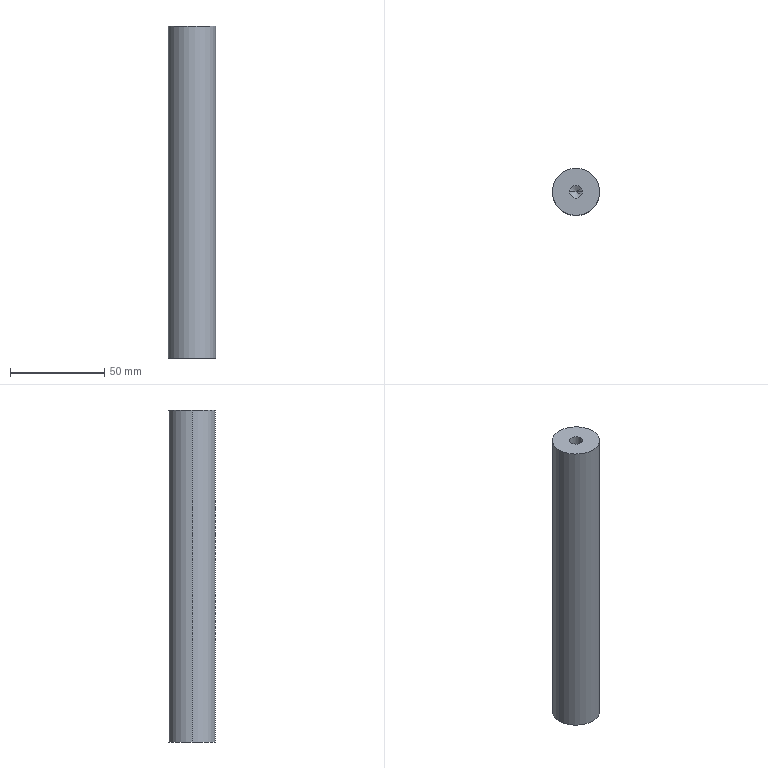Part | SolidWorks | features HoleWzd 2, Extrusion 1 | 1 solid | 12 faces | box 25 x 25 x 176 mm | volume 84910 mm3 | cylinder 6 | cone 4 | plane 2 | commonest cylinder face diameters 6.8 x4 25 x2
STEP:
#1=CARTESIAN_POINT('',(-3.4,0.,156.25));
#2=VERTEX_POINT('',#1);
#3=CARTESIAN_POINT('',(3.4,0.,156.25));
#4=VERTEX_POINT('',#3);
#5=CARTESIAN_POINT('',(0.,0.,156.25));
#6=DIRECTION('',(0.,0.,1.));
#7=DIRECTION('',(1.,0.,0.));
#8=AXIS2_PLACEMENT_3D('',#5,#6,#7);
#9=CIRCLE('',#8,3.4);
#10=EDGE_CURVE('',#2,#4,#9,.T.);
#11=ORIENTED_EDGE('',*,*,#10,.F.);
#12=CARTESIAN_POINT('',(-3.4,0.,176.));
#13=VERTEX_POINT('',#12);
#14=CARTESIAN_POINT('',(-3.4,0.,176.));
#15=DIRECTION('',(0.,0.,1.));
#16=VECTOR('',#15,1000.);
#17=LINE('',#14,#16);
#18=EDGE_CURVE('',#2,#13,#17,.T.);
#19=ORIENTED_EDGE('',*,*,#18,.T.);
#20=CARTESIAN_POINT('',(3.4,0.,176.));
#21=VERTEX_POINT('',#20);
#22=CARTESIAN_POINT('',(0.,0.,176.));
#23=DIRECTION('',(0.,0.,1.));
#24=DIRECTION('',(1.,0.,0.));
#25=AXIS2_PLACEMENT_3D('',#22,#23,#24);
#26=CIRCLE('',#25,3.4);
#27=EDGE_CURVE('',#13,#21,#26,.T.);
#28=ORIENTED_EDGE('',*,*,#27,.T.);
#29=CARTESIAN_POINT('',(3.4,0.,176.));
#30=DIRECTION('',(0.,0.,1.));
#31=VECTOR('',#30,1000.);
#32=LINE('',#29,#31);
#33=EDGE_CURVE('',#4,#21,#32,.T.);
#34=ORIENTED_EDGE('',*,*,#33,.F.);
#35=EDGE_LOOP('',(#11,#19,#28,#34));
#36=FACE_OUTER_BOUND('',#35,.T.);
#37=CARTESIAN_POINT('',(0.,0.,176.));
#38=DIRECTION('',(0.,0.,1.));
#39=DIRECTION('',(1.,0.,0.));
#40=AXIS2_PLACEMENT_3D('',#37,#38,#39);
#41=CYLINDRICAL_SURFACE('',#40,3.4);
#42=ADVANCED_FACE('',(#36),#41,.F.);
#43=CARTESIAN_POINT('',(0.,0.,154.207));
#44=VERTEX_POINT('',#43);
#45=CARTESIAN_POINT('',(3.4,0.,156.25));
#46=DIRECTION('',(0.8572,0.,0.515));
#47=VECTOR('',#46,1000.);
#48=LINE('',#45,#47);
#49=EDGE_CURVE('',#44,#4,#48,.T.);
#50=ORIENTED_EDGE('',*,*,#49,.F.);
#51=CARTESIAN_POINT('',(-3.4,0.,156.25));
#52=DIRECTION('',(-0.8572,0.,0.515));
#53=VECTOR('',#52,1000.);
#54=LINE('',#51,#53);
#55=EDGE_CURVE('',#44,#2,#54,.T.);
#56=ORIENTED_EDGE('',*,*,#55,.T.);
#57=ORIENTED_EDGE('',*,*,#10,.T.);
#58=EDGE_LOOP('',(#50,#56,#57));
#59=FACE_OUTER_BOUND('',#58,.T.);
#60=CARTESIAN_POINT('',(0.,0.,156.25));
#61=DIRECTION('',(0.,0.,1.));
#62=DIRECTION('',(1.,0.,0.));
#63=AXIS2_PLACEMENT_3D('',#60,#61,#62);
#64=CONICAL_SURFACE('',#63,3.4,1.03);
#65=ADVANCED_FACE('',(#59),#64,.F.);
#66=CARTESIAN_POINT('',(3.4,0.,19.75));
#67=VERTEX_POINT('',#66);
#68=CARTESIAN_POINT('',(-3.4,0.,19.75));
#69=VERTEX_POINT('',#68);
#70=CARTESIAN_POINT('',(0.,0.,19.75));
#71=DIRECTION('',(0.,0.,-1.));
#72=DIRECTION('',(-1.,0.,0.));
#73=AXIS2_PLACEMENT_3D('',#70,#71,#72);
#74=CIRCLE('',#73,3.4);
#75=EDGE_CURVE('',#67,#69,#74,.T.);
#76=ORIENTED_EDGE('',*,*,#75,.F.);
#77=CARTESIAN_POINT('',(3.4,0.,0.));
#78=VERTEX_POINT('',#77);
#79=CARTESIAN_POINT('',(3.4,0.,0.));
#80=DIRECTION('',(0.,0.,-1.));
#81=VECTOR('',#80,1000.);
#82=LINE('',#79,#81);
#83=EDGE_CURVE('',#67,#78,#82,.T.);
#84=ORIENTED_EDGE('',*,*,#83,.T.);
#85=CARTESIAN_POINT('',(-3.4,0.,0.));
#86=VERTEX_POINT('',#85);
#87=CARTESIAN_POINT('',(0.,0.,0.));
#88=DIRECTION('',(0.,0.,-1.));
#89=DIRECTION('',(-1.,0.,0.));
#90=AXIS2_PLACEMENT_3D('',#87,#88,#89);
#91=CIRCLE('',#90,3.4);
#92=EDGE_CURVE('',#78,#86,#91,.T.);
#93=ORIENTED_EDGE('',*,*,#92,.T.);
#94=CARTESIAN_POINT('',(-3.4,0.,0.));
#95=DIRECTION('',(0.,0.,-1.));
#96=VECTOR('',#95,1000.);
#97=LINE('',#94,#96);
#98=EDGE_CURVE('',#69,#86,#97,.T.);
#99=ORIENTED_EDGE('',*,*,#98,.F.);
#100=EDGE_LOOP('',(#76,#84,#93,#99));
#101=FACE_OUTER_BOUND('',#100,.T.);
#102=CARTESIAN_POINT('',(0.,0.,0.));
#103=DIRECTION('',(0.,0.,-1.));
#104=DIRECTION('',(-1.,0.,0.));
#105=AXIS2_PLACEMENT_3D('',#102,#103,#104);
#106=CYLINDRICAL_SURFACE('',#105,3.4);
#107=ADVANCED_FACE('',(#101),#106,.F.);
#108=CARTESIAN_POINT('',(0.,0.,21.793));
#109=VERTEX_POINT('',#108);
#110=CARTESIAN_POINT('',(-3.4,0.,19.75));
#111=DIRECTION('',(-0.8572,0.,-0.515));
#112=VECTOR('',#111,1000.);
#113=LINE('',#110,#112);
#114=EDGE_CURVE('',#109,#69,#113,.T.);
#115=ORIENTED_EDGE('',*,*,#114,.F.);
#116=CARTESIAN_POINT('',(3.4,0.,19.75));
#117=DIRECTION('',(0.8572,0.,-0.515));
#118=VECTOR('',#117,1000.);
#119=LINE('',#116,#118);
#120=EDGE_CURVE('',#109,#67,#119,.T.);
#121=ORIENTED_EDGE('',*,*,#120,.T.);
#122=ORIENTED_EDGE('',*,*,#75,.T.);
#123=EDGE_LOOP('',(#115,#121,#122));
#124=FACE_OUTER_BOUND('',#123,.T.);
#125=CARTESIAN_POINT('',(0.,0.,19.75));
#126=DIRECTION('',(0.,0.,-1.));
#127=DIRECTION('',(-1.,0.,0.));
#128=AXIS2_PLACEMENT_3D('',#125,#126,#127);
#129=CONICAL_SURFACE('',#128,3.4,1.03);
#130=ADVANCED_FACE('',(#124),#129,.F.);
#131=CARTESIAN_POINT('',(12.5,0.,176.));
#132=VERTEX_POINT('',#131);
#133=CARTESIAN_POINT('',(-12.5,0.,176.));
#134=VERTEX_POINT('',#133);
#135=CARTESIAN_POINT('',(0.,0.,176.));
#136=DIRECTION('',(0.,0.,1.));
#137=DIRECTION('',(1.,0.,0.));
#138=AXIS2_PLACEMENT_3D('',#135,#136,#137);
#139=CIRCLE('',#138,12.5);
#140=EDGE_CURVE('',#132,#134,#139,.T.);
#141=ORIENTED_EDGE('',*,*,#140,.F.);
#142=CARTESIAN_POINT('',(12.5,0.,0.));
#143=VERTEX_POINT('',#142);
#144=CARTESIAN_POINT('',(12.5,0.,176.));
#145=DIRECTION('',(0.,0.,-1.));
#146=VECTOR('',#145,1000.);
#147=LINE('',#144,#146);
#148=EDGE_CURVE('',#132,#143,#147,.T.);
#149=ORIENTED_EDGE('',*,*,#148,.T.);
#150=CARTESIAN_POINT('',(-12.5,0.,0.));
#151=VERTEX_POINT('',#150);
#152=CARTESIAN_POINT('',(0.,0.,0.));
#153=DIRECTION('',(0.,0.,1.));
#154=DIRECTION('',(1.,0.,0.));
#155=AXIS2_PLACEMENT_3D('',#152,#153,#154);
#156=CIRCLE('',#155,12.5);
#157=EDGE_CURVE('',#143,#151,#156,.T.);
#158=ORIENTED_EDGE('',*,*,#157,.T.);
#159=CARTESIAN_POINT('',(-12.5,0.,176.));
#160=DIRECTION('',(0.,0.,-1.));
#161=VECTOR('',#160,1000.);
#162=LINE('',#159,#161);
#163=EDGE_CURVE('',#134,#151,#162,.T.);
#164=ORIENTED_EDGE('',*,*,#163,.F.);
#165=EDGE_LOOP('',(#141,#149,#158,#164));
#166=FACE_OUTER_BOUND('',#165,.T.);
#167=CARTESIAN_POINT('',(0.,0.,176.));
#168=DIRECTION('',(0.,0.,-1.));
#169=DIRECTION('',(-1.,0.,0.));
#170=AXIS2_PLACEMENT_3D('',#167,#168,#169);
#171=CYLINDRICAL_SURFACE('',#170,12.5);
#172=ADVANCED_FACE('',(#166),#171,.T.);
#173=ORIENTED_EDGE('',*,*,#148,.F.);
#174=CARTESIAN_POINT('',(0.,0.,176.));
#175=DIRECTION('',(0.,0.,1.));
#176=DIRECTION('',(1.,0.,0.));
#177=AXIS2_PLACEMENT_3D('',#174,#175,#176);
#178=CIRCLE('',#177,12.5);
#179=EDGE_CURVE('',#134,#132,#178,.T.);
#180=ORIENTED_EDGE('',*,*,#179,.F.);
#181=ORIENTED_EDGE('',*,*,#163,.T.);
#182=CARTESIAN_POINT('',(0.,0.,0.));
#183=DIRECTION('',(0.,0.,1.));
#184=DIRECTION('',(1.,0.,0.));
#185=AXIS2_PLACEMENT_3D('',#182,#183,#184);
#186=CIRCLE('',#185,12.5);
#187=EDGE_CURVE('',#151,#143,#186,.T.);
#188=ORIENTED_EDGE('',*,*,#187,.T.);
#189=EDGE_LOOP('',(#173,#180,#181,#188));
#190=FACE_OUTER_BOUND('',#189,.T.);
#191=CARTESIAN_POINT('',(0.,0.,176.));
#192=DIRECTION('',(0.,0.,-1.));
#193=DIRECTION('',(-1.,0.,0.));
#194=AXIS2_PLACEMENT_3D('',#191,#192,#193);
#195=CYLINDRICAL_SURFACE('',#194,12.5);
#196=ADVANCED_FACE('',(#190),#195,.T.);
#197=CARTESIAN_POINT('',(0.,0.,176.));
#198=DIRECTION('',(0.,0.,1.));
#199=DIRECTION('',(1.,0.,0.));
#200=AXIS2_PLACEMENT_3D('',#197,#198,#199);
#201=CIRCLE('',#200,3.4);
#202=EDGE_CURVE('',#21,#13,#201,.T.);
#203=ORIENTED_EDGE('',*,*,#202,.F.);
#204=ORIENTED_EDGE('',*,*,#27,.F.);
#205=EDGE_LOOP('',(#203,#204));
#206=FACE_BOUND('',#205,.T.);
#207=ORIENTED_EDGE('',*,*,#179,.T.);
#208=ORIENTED_EDGE('',*,*,#140,.T.);
#209=EDGE_LOOP('',(#207,#208));
#210=FACE_OUTER_BOUND('',#209,.T.);
#211=CARTESIAN_POINT('',(0.,0.,176.));
#212=DIRECTION('',(0.,0.,1.));
#213=DIRECTION('',(1.,0.,0.));
#214=AXIS2_PLACEMENT_3D('',#211,#212,#213);
#215=PLANE('',#214);
#216=ADVANCED_FACE('',(#206,#210),#215,.T.);
#217=CARTESIAN_POINT('',(0.,0.,0.));
#218=DIRECTION('',(0.,0.,-1.));
#219=DIRECTION('',(-1.,0.,0.));
#220=AXIS2_PLACEMENT_3D('',#217,#218,#219);
#221=CIRCLE('',#220,3.4);
#222=EDGE_CURVE('',#86,#78,#221,.T.);
#223=ORIENTED_EDGE('',*,*,#222,.F.);
#224=ORIENTED_EDGE('',*,*,#92,.F.);
#225=EDGE_LOOP('',(#223,#224));
#226=FACE_BOUND('',#225,.T.);
#227=ORIENTED_EDGE('',*,*,#187,.F.);
#228=ORIENTED_EDGE('',*,*,#157,.F.);
#229=EDGE_LOOP('',(#227,#228));
#230=FACE_OUTER_BOUND('',#229,.T.);
#231=CARTESIAN_POINT('',(0.,0.,0.));
#232=DIRECTION('',(0.,0.,1.));
#233=DIRECTION('',(1.,0.,0.));
#234=AXIS2_PLACEMENT_3D('',#231,#232,#233);
#235=PLANE('',#234);
#236=ADVANCED_FACE('',(#226,#230),#235,.F.);
#237=ORIENTED_EDGE('',*,*,#120,.F.);
#238=ORIENTED_EDGE('',*,*,#114,.T.);
#239=CARTESIAN_POINT('',(0.,0.,19.75));
#240=DIRECTION('',(0.,0.,-1.));
#241=DIRECTION('',(-1.,0.,0.));
#242=AXIS2_PLACEMENT_3D('',#239,#240,#241);
#243=CIRCLE('',#242,3.4);
#244=EDGE_CURVE('',#69,#67,#243,.T.);
#245=ORIENTED_EDGE('',*,*,#244,.T.);
#246=EDGE_LOOP('',(#237,#238,#245));
#247=FACE_OUTER_BOUND('',#246,.T.);
#248=CARTESIAN_POINT('',(0.,0.,19.75));
#249=DIRECTION('',(0.,0.,-1.));
#250=DIRECTION('',(-1.,0.,0.));
#251=AXIS2_PLACEMENT_3D('',#248,#249,#250);
#252=CONICAL_SURFACE('',#251,3.4,1.03);
#253=ADVANCED_FACE('',(#247),#252,.F.);
#254=ORIENTED_EDGE('',*,*,#83,.F.);
#255=ORIENTED_EDGE('',*,*,#244,.F.);
#256=ORIENTED_EDGE('',*,*,#98,.T.);
#257=ORIENTED_EDGE('',*,*,#222,.T.);
#258=EDGE_LOOP('',(#254,#255,#256,#257));
#259=FACE_OUTER_BOUND('',#258,.T.);
#260=CARTESIAN_POINT('',(0.,0.,0.));
#261=DIRECTION('',(0.,0.,-1.));
#262=DIRECTION('',(-1.,0.,0.));
#263=AXIS2_PLACEMENT_3D('',#260,#261,#262);
#264=CYLINDRICAL_SURFACE('',#263,3.4);
#265=ADVANCED_FACE('',(#259),#264,.F.);
#266=ORIENTED_EDGE('',*,*,#55,.F.);
#267=ORIENTED_EDGE('',*,*,#49,.T.);
#268=CARTESIAN_POINT('',(0.,0.,156.25));
#269=DIRECTION('',(0.,0.,1.));
#270=DIRECTION('',(1.,0.,0.));
#271=AXIS2_PLACEMENT_3D('',#268,#269,#270);
#272=CIRCLE('',#271,3.4);
#273=EDGE_CURVE('',#4,#2,#272,.T.);
#274=ORIENTED_EDGE('',*,*,#273,.T.);
#275=EDGE_LOOP('',(#266,#267,#274));
#276=FACE_OUTER_BOUND('',#275,.T.);
#277=CARTESIAN_POINT('',(0.,0.,156.25));
#278=DIRECTION('',(0.,0.,1.));
#279=DIRECTION('',(1.,0.,0.));
#280=AXIS2_PLACEMENT_3D('',#277,#278,#279);
#281=CONICAL_SURFACE('',#280,3.4,1.03);
#282=ADVANCED_FACE('',(#276),#281,.F.);
#283=ORIENTED_EDGE('',*,*,#18,.F.);
#284=ORIENTED_EDGE('',*,*,#273,.F.);
#285=ORIENTED_EDGE('',*,*,#33,.T.);
#286=ORIENTED_EDGE('',*,*,#202,.T.);
#287=EDGE_LOOP('',(#283,#284,#285,#286));
#288=FACE_OUTER_BOUND('',#287,.T.);
#289=CARTESIAN_POINT('',(0.,0.,176.));
#290=DIRECTION('',(0.,0.,1.));
#291=DIRECTION('',(1.,0.,0.));
#292=AXIS2_PLACEMENT_3D('',#289,#290,#291);
#293=CYLINDRICAL_SURFACE('',#292,3.4);
#294=ADVANCED_FACE('',(#288),#293,.F.);
#295=CLOSED_SHELL('',(#42,#65,#107,#130,#172,#196,#216,#236,#253,#265,#282,#294));
#296=MANIFOLD_SOLID_BREP('',#295);
#297=CARTESIAN_POINT('',(0.,0.,0.));
#298=DIRECTION('',(0.,0.,1.));
#299=DIRECTION('',(1.,0.,0.));
#300=AXIS2_PLACEMENT_3D('',#297,#298,#299);
#301=(LENGTH_UNIT()NAMED_UNIT(*)SI_UNIT(.MILLI.,.METRE.));
#302=UNCERTAINTY_MEASURE_WITH_UNIT(LENGTH_MEASURE(0.00001),#301,'','');
#303=(NAMED_UNIT(*)PLANE_ANGLE_UNIT()SI_UNIT($,.RADIAN.));
#304=(NAMED_UNIT(*)SI_UNIT($,.STERADIAN.)SOLID_ANGLE_UNIT());
#305=(GEOMETRIC_REPRESENTATION_CONTEXT(3)GLOBAL_UNCERTAINTY_ASSIGNED_CONTEXT((#302))GLOBAL_UNIT_ASSIGNED_CONTEXT((#301,#303,#304))REPRESENTATION_CONTEXT('',''));
#306=ADVANCED_BREP_SHAPE_REPRESENTATION('',(#296,#300),#305);